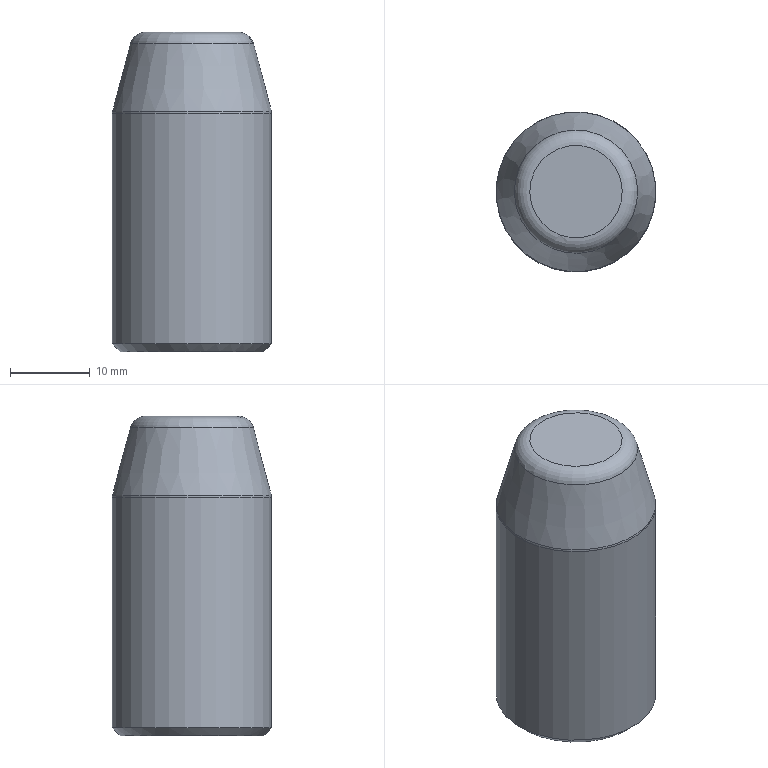Part | STEP file | SN10_014_001_PINO | 1 solid | 9 faces | box 20 x 20 x 40 mm | volume 11102 mm3 | cone 3 | plane 2 | torus 2 | cylinder 2 | commonest cylinder face diameters 6.647 x1 20 x1
STEP:
#1=CARTESIAN_POINT('',(0.,0.,0.));
#2=DIRECTION('',(0.,0.,1.));
#3=DIRECTION('',(1.,0.,0.));
#4=AXIS2_PLACEMENT_3D('',#1,#2,#3);
#5=CARTESIAN_POINT('',(2.917,1.593,47.));
#6=VERTEX_POINT('',#5);
#7=CARTESIAN_POINT('',(0.,0.,47.));
#8=DIRECTION('',(0.,0.,-1.));
#9=DIRECTION('',(1.,0.,0.));
#10=AXIS2_PLACEMENT_3D('',#7,#8,#9);
#11=CIRCLE('',#10,3.324);
#12=CARTESIAN_POINT('',(0.,0.,48.341));
#13=DIRECTION('',(0.,0.,-1.));
#14=DIRECTION('',(0.8776,0.4794,0.));
#15=AXIS2_PLACEMENT_3D('',#12,#13,#14);
#16=CONICAL_SURFACE('',#15,1.,1.047);
#17=CARTESIAN_POINT('',(-5.783,1.341));
#18=DIRECTION('',(1.,0.));
#19=VECTOR('',#18,1.);
#20=LINE('',#17,#19);
#21=(GEOMETRIC_REPRESENTATION_CONTEXT(2)PARAMETRIC_REPRESENTATION_CONTEXT()REPRESENTATION_CONTEXT('',''));
#22=DEFINITIONAL_REPRESENTATION('',(#20),#21);
#23=PCURVE('',#16,#22);
#24=CARTESIAN_POINT('',(0.,0.,29.1));
#25=DIRECTION('',(0.,0.,1.));
#26=DIRECTION('',(0.8776,0.4794,0.));
#27=AXIS2_PLACEMENT_3D('',#24,#25,#26);
#28=CYLINDRICAL_SURFACE('',#27,3.324);
#29=CARTESIAN_POINT('',(12.066,17.9));
#30=DIRECTION('',(-1.,0.));
#31=VECTOR('',#30,1.);
#32=LINE('',#29,#31);
#33=(GEOMETRIC_REPRESENTATION_CONTEXT(2)PARAMETRIC_REPRESENTATION_CONTEXT()REPRESENTATION_CONTEXT('',''));
#34=DEFINITIONAL_REPRESENTATION('',(#32),#33);
#35=PCURVE('',#28,#34);
#36=SURFACE_CURVE('',#11,(#23,#35),.PCURVE_S1.);
#37=EDGE_CURVE('',#6,#6,#36,.T.);
#38=ORIENTED_EDGE('',*,*,#37,.F.);
#39=CARTESIAN_POINT('',(0.,0.,48.919));
#40=VERTEX_POINT('',#39);
#41=CARTESIAN_POINT('',(0.,0.,48.919));
#42=CARTESIAN_POINT('',(2.917,1.593,47.));
#43=B_SPLINE_CURVE_WITH_KNOTS('',1,(#41,#42),.UNSPECIFIED.,.F.,.F.,(2,2),(-1.155,2.683),.PIECEWISE_BEZIER_KNOTS.);
#44=CARTESIAN_POINT('',(0.,0.));
#45=DIRECTION('',(0.,1.));
#46=VECTOR('',#45,1.);
#47=LINE('',#44,#46);
#48=(GEOMETRIC_REPRESENTATION_CONTEXT(2)PARAMETRIC_REPRESENTATION_CONTEXT()REPRESENTATION_CONTEXT('',''));
#49=DEFINITIONAL_REPRESENTATION('',(#47),#48);
#50=PCURVE('',#16,#49);
#51=CARTESIAN_POINT('',(6.283,0.));
#52=DIRECTION('',(0.,1.));
#53=VECTOR('',#52,1.);
#54=LINE('',#51,#53);
#55=(GEOMETRIC_REPRESENTATION_CONTEXT(2)PARAMETRIC_REPRESENTATION_CONTEXT()REPRESENTATION_CONTEXT('',''));
#56=DEFINITIONAL_REPRESENTATION('',(#54),#55);
#57=PCURVE('',#16,#56);
#58=SEAM_CURVE('',#43,(#50,#57),.PCURVE_S1.);
#59=EDGE_CURVE('',#40,#6,#58,.T.);
#60=ORIENTED_EDGE('',*,*,#59,.F.);
#61=ORIENTED_EDGE('',*,*,#59,.T.);
#62=EDGE_LOOP('',(#38,#60,#61));
#63=FACE_BOUND('',#62,.F.);
#64=ADVANCED_FACE('',(#63),#16,.F.);
#65=CARTESIAN_POINT('',(5.078,2.774,69.));
#66=VERTEX_POINT('',#65);
#67=CARTESIAN_POINT('',(0.,0.,69.));
#68=DIRECTION('',(0.,0.,1.));
#69=DIRECTION('',(1.,0.,0.));
#70=AXIS2_PLACEMENT_3D('',#67,#68,#69);
#71=CIRCLE('',#70,5.786);
#72=CARTESIAN_POINT('',(7.321,0.,69.));
#73=DIRECTION('',(0.,0.,1.));
#74=DIRECTION('',(1.,0.,0.));
#75=AXIS2_PLACEMENT_3D('',#72,#73,#74);
#76=PLANE('',#75);
#77=CARTESIAN_POINT('',(-7.321,0.));
#78=DIRECTION('',(1.,0.));
#79=AXIS2_PLACEMENT_2D('',#77,#78);
#80=CIRCLE('',#79,5.786);
#81=(GEOMETRIC_REPRESENTATION_CONTEXT(2)PARAMETRIC_REPRESENTATION_CONTEXT()REPRESENTATION_CONTEXT('',''));
#82=DEFINITIONAL_REPRESENTATION('',(#80),#81);
#83=PCURVE('',#76,#82);
#84=CARTESIAN_POINT('',(0.,0.,67.));
#85=DIRECTION('',(0.,0.,1.));
#86=DIRECTION('',(1.,0.,0.));
#87=AXIS2_PLACEMENT_3D('',#84,#85,#86);
#88=TOROIDAL_SURFACE('',#87,5.786,2.);
#89=CARTESIAN_POINT('',(0.,7.854));
#90=DIRECTION('',(1.,0.));
#91=VECTOR('',#90,1.);
#92=LINE('',#89,#91);
#93=(GEOMETRIC_REPRESENTATION_CONTEXT(2)PARAMETRIC_REPRESENTATION_CONTEXT()REPRESENTATION_CONTEXT('',''));
#94=DEFINITIONAL_REPRESENTATION('',(#92),#93);
#95=PCURVE('',#88,#94);
#96=SURFACE_CURVE('',#71,(#83,#95),.PCURVE_S1.);
#97=EDGE_CURVE('',#66,#66,#96,.T.);
#98=ORIENTED_EDGE('',*,*,#97,.T.);
#99=EDGE_LOOP('',(#98));
#100=FACE_BOUND('',#99,.T.);
#101=ADVANCED_FACE('',(#100),#76,.T.);
#102=ORIENTED_EDGE('',*,*,#97,.F.);
#103=CARTESIAN_POINT('',(6.773,3.7,67.518));
#104=VERTEX_POINT('',#103);
#105=CARTESIAN_POINT('',(6.773,3.7,67.518));
#106=CARTESIAN_POINT('',(6.672,3.645,67.945));
#107=CARTESIAN_POINT('',(6.475,3.537,68.335));
#108=CARTESIAN_POINT('',(6.193,3.383,68.656));
#109=CARTESIAN_POINT('',(5.848,3.195,68.883));
#110=CARTESIAN_POINT('',(5.466,2.986,69.));
#111=CARTESIAN_POINT('',(5.078,2.774,69.));
#112=(BOUNDED_CURVE()B_SPLINE_CURVE(6,(#105,#106,#107,#108,#109,#110,#111),.UNSPECIFIED.,.F.,.F.)B_SPLINE_CURVE_WITH_KNOTS((7,7),(0.2618,1.571),.PIECEWISE_BEZIER_KNOTS.)CURVE()GEOMETRIC_REPRESENTATION_ITEM()RATIONAL_B_SPLINE_CURVE((1.022,1.007,0.9986,0.9958,0.9986,1.007,1.022))REPRESENTATION_ITEM(''));
#113=CARTESIAN_POINT('',(0.5,6.283));
#114=DIRECTION('',(0.,1.));
#115=VECTOR('',#114,1.);
#116=LINE('',#113,#115);
#117=(GEOMETRIC_REPRESENTATION_CONTEXT(2)PARAMETRIC_REPRESENTATION_CONTEXT()REPRESENTATION_CONTEXT('',''));
#118=DEFINITIONAL_REPRESENTATION('',(#116),#117);
#119=PCURVE('',#88,#118);
#120=CARTESIAN_POINT('',(6.783,6.283));
#121=DIRECTION('',(0.,1.));
#122=VECTOR('',#121,1.);
#123=LINE('',#120,#122);
#124=(GEOMETRIC_REPRESENTATION_CONTEXT(2)PARAMETRIC_REPRESENTATION_CONTEXT()REPRESENTATION_CONTEXT('',''));
#125=DEFINITIONAL_REPRESENTATION('',(#123),#124);
#126=PCURVE('',#88,#125);
#127=SEAM_CURVE('',#112,(#119,#126),.PCURVE_S1.);
#128=EDGE_CURVE('',#104,#66,#127,.T.);
#129=ORIENTED_EDGE('',*,*,#128,.F.);
#130=CARTESIAN_POINT('',(0.,0.,67.518));
#131=DIRECTION('',(0.,0.,1.));
#132=DIRECTION('',(1.,0.,0.));
#133=AXIS2_PLACEMENT_3D('',#130,#131,#132);
#134=CIRCLE('',#133,7.718);
#135=CARTESIAN_POINT('',(0.,6.545));
#136=DIRECTION('',(1.,0.));
#137=VECTOR('',#136,1.);
#138=LINE('',#135,#137);
#139=(GEOMETRIC_REPRESENTATION_CONTEXT(2)PARAMETRIC_REPRESENTATION_CONTEXT()REPRESENTATION_CONTEXT('',''));
#140=DEFINITIONAL_REPRESENTATION('',(#138),#139);
#141=PCURVE('',#88,#140);
#142=CARTESIAN_POINT('',(0.,0.,69.));
#143=DIRECTION('',(0.,0.,-1.));
#144=DIRECTION('',(0.8776,0.4794,0.));
#145=AXIS2_PLACEMENT_3D('',#142,#143,#144);
#146=CONICAL_SURFACE('',#145,7.321,0.2618);
#147=CARTESIAN_POINT('',(6.783,1.482));
#148=DIRECTION('',(-1.,0.));
#149=VECTOR('',#148,1.);
#150=LINE('',#147,#149);
#151=(GEOMETRIC_REPRESENTATION_CONTEXT(2)PARAMETRIC_REPRESENTATION_CONTEXT()REPRESENTATION_CONTEXT('',''));
#152=DEFINITIONAL_REPRESENTATION('',(#150),#151);
#153=PCURVE('',#146,#152);
#154=SURFACE_CURVE('',#134,(#141,#153),.PCURVE_S1.);
#155=EDGE_CURVE('',#104,#104,#154,.T.);
#156=ORIENTED_EDGE('',*,*,#155,.T.);
#157=ORIENTED_EDGE('',*,*,#128,.T.);
#158=EDGE_LOOP('',(#102,#129,#156,#157));
#159=FACE_BOUND('',#158,.T.);
#160=ADVANCED_FACE('',(#159),#88,.T.);
#161=CARTESIAN_POINT('',(8.746,4.778,59.127));
#162=VERTEX_POINT('',#161);
#163=CARTESIAN_POINT('',(-8.746,-4.778,59.127));
#164=VERTEX_POINT('',#163);
#165=CARTESIAN_POINT('',(0.,0.,59.127));
#166=DIRECTION('',(0.,0.,-1.));
#167=DIRECTION('',(1.,0.,0.));
#168=AXIS2_PLACEMENT_3D('',#165,#166,#167);
#169=CIRCLE('',#168,9.966);
#170=CARTESIAN_POINT('',(-5.783,9.873));
#171=DIRECTION('',(1.,0.));
#172=VECTOR('',#171,1.);
#173=LINE('',#170,#172);
#174=(GEOMETRIC_REPRESENTATION_CONTEXT(2)PARAMETRIC_REPRESENTATION_CONTEXT()REPRESENTATION_CONTEXT('',''));
#175=DEFINITIONAL_REPRESENTATION('',(#173),#174);
#176=PCURVE('',#146,#175);
#177=CARTESIAN_POINT('',(0.,0.,58.868));
#178=DIRECTION('',(0.,0.,-1.));
#179=DIRECTION('',(-1.,0.,0.));
#180=AXIS2_PLACEMENT_3D('',#177,#178,#179);
#181=TOROIDAL_SURFACE('',#180,9.,1.);
#182=CARTESIAN_POINT('',(-3.142,6.021));
#183=DIRECTION('',(1.,0.));
#184=VECTOR('',#183,1.);
#185=LINE('',#182,#184);
#186=(GEOMETRIC_REPRESENTATION_CONTEXT(2)PARAMETRIC_REPRESENTATION_CONTEXT()REPRESENTATION_CONTEXT('',''));
#187=DEFINITIONAL_REPRESENTATION('',(#185),#186);
#188=PCURVE('',#181,#187);
#189=SURFACE_CURVE('',#169,(#176,#188),.PCURVE_S1.);
#190=EDGE_CURVE('',#162,#164,#189,.T.);
#191=ORIENTED_EDGE('',*,*,#190,.F.);
#192=CARTESIAN_POINT('',(6.773,3.7,67.518));
#193=CARTESIAN_POINT('',(8.746,4.778,59.127));
#194=B_SPLINE_CURVE_WITH_KNOTS('',1,(#192,#193),.UNSPECIFIED.,.F.,.F.,(2,2),(1.535,10.221),.PIECEWISE_BEZIER_KNOTS.);
#195=CARTESIAN_POINT('',(0.,0.));
#196=DIRECTION('',(0.,1.));
#197=VECTOR('',#196,1.);
#198=LINE('',#195,#197);
#199=(GEOMETRIC_REPRESENTATION_CONTEXT(2)PARAMETRIC_REPRESENTATION_CONTEXT()REPRESENTATION_CONTEXT('',''));
#200=DEFINITIONAL_REPRESENTATION('',(#198),#199);
#201=PCURVE('',#146,#200);
#202=CARTESIAN_POINT('',(6.283,0.));
#203=DIRECTION('',(0.,1.));
#204=VECTOR('',#203,1.);
#205=LINE('',#202,#204);
#206=(GEOMETRIC_REPRESENTATION_CONTEXT(2)PARAMETRIC_REPRESENTATION_CONTEXT()REPRESENTATION_CONTEXT('',''));
#207=DEFINITIONAL_REPRESENTATION('',(#205),#206);
#208=PCURVE('',#146,#207);
#209=SEAM_CURVE('',#194,(#201,#208),.PCURVE_S1.);
#210=EDGE_CURVE('',#104,#162,#209,.T.);
#211=ORIENTED_EDGE('',*,*,#210,.F.);
#212=ORIENTED_EDGE('',*,*,#155,.F.);
#213=ORIENTED_EDGE('',*,*,#210,.T.);
#214=CARTESIAN_POINT('',(0.,0.,59.127));
#215=DIRECTION('',(0.,0.,-1.));
#216=DIRECTION('',(1.,0.,0.));
#217=AXIS2_PLACEMENT_3D('',#214,#215,#216);
#218=CIRCLE('',#217,9.966);
#219=CARTESIAN_POINT('',(0.5,9.873));
#220=DIRECTION('',(1.,0.));
#221=VECTOR('',#220,1.);
#222=LINE('',#219,#221);
#223=(GEOMETRIC_REPRESENTATION_CONTEXT(2)PARAMETRIC_REPRESENTATION_CONTEXT()REPRESENTATION_CONTEXT('',''));
#224=DEFINITIONAL_REPRESENTATION('',(#222),#223);
#225=PCURVE('',#146,#224);
#226=CARTESIAN_POINT('',(3.142,6.021));
#227=DIRECTION('',(1.,0.));
#228=VECTOR('',#227,1.);
#229=LINE('',#226,#228);
#230=(GEOMETRIC_REPRESENTATION_CONTEXT(2)PARAMETRIC_REPRESENTATION_CONTEXT()REPRESENTATION_CONTEXT('',''));
#231=DEFINITIONAL_REPRESENTATION('',(#229),#230);
#232=PCURVE('',#181,#231);
#233=SURFACE_CURVE('',#218,(#225,#232),.PCURVE_S1.);
#234=EDGE_CURVE('',#164,#162,#233,.T.);
#235=ORIENTED_EDGE('',*,*,#234,.F.);
#236=EDGE_LOOP('',(#191,#211,#212,#213,#235));
#237=FACE_BOUND('',#236,.T.);
#238=ADVANCED_FACE('',(#237),#146,.T.);
#239=ORIENTED_EDGE('',*,*,#234,.T.);
#240=CARTESIAN_POINT('',(8.776,4.794,58.868));
#241=VERTEX_POINT('',#240);
#242=CARTESIAN_POINT('',(8.746,4.778,59.127));
#243=CARTESIAN_POINT('',(8.756,4.783,59.085));
#244=CARTESIAN_POINT('',(8.764,4.788,59.042));
#245=CARTESIAN_POINT('',(8.77,4.791,58.999));
#246=CARTESIAN_POINT('',(8.774,4.793,58.956));
#247=CARTESIAN_POINT('',(8.776,4.794,58.912));
#248=CARTESIAN_POINT('',(8.776,4.794,58.868));
#249=(BOUNDED_CURVE()B_SPLINE_CURVE(6,(#242,#243,#244,#245,#246,#247,#248),.UNSPECIFIED.,.F.,.F.)B_SPLINE_CURVE_WITH_KNOTS((7,7),(6.021,6.283),.PIECEWISE_BEZIER_KNOTS.)CURVE()GEOMETRIC_REPRESENTATION_ITEM()RATIONAL_B_SPLINE_CURVE((1.001,1.,0.9999,0.9998,0.9999,1.,1.001))REPRESENTATION_ITEM(''));
#250=CARTESIAN_POINT('',(8.925,0.));
#251=DIRECTION('',(0.,1.));
#252=VECTOR('',#251,1.);
#253=LINE('',#250,#252);
#254=(GEOMETRIC_REPRESENTATION_CONTEXT(2)PARAMETRIC_REPRESENTATION_CONTEXT()REPRESENTATION_CONTEXT('',''));
#255=DEFINITIONAL_REPRESENTATION('',(#253),#254);
#256=PCURVE('',#181,#255);
#257=CARTESIAN_POINT('',(2.642,0.));
#258=DIRECTION('',(0.,1.));
#259=VECTOR('',#258,1.);
#260=LINE('',#257,#259);
#261=(GEOMETRIC_REPRESENTATION_CONTEXT(2)PARAMETRIC_REPRESENTATION_CONTEXT()REPRESENTATION_CONTEXT('',''));
#262=DEFINITIONAL_REPRESENTATION('',(#260),#261);
#263=PCURVE('',#181,#262);
#264=SEAM_CURVE('',#249,(#256,#263),.PCURVE_S1.);
#265=EDGE_CURVE('',#162,#241,#264,.T.);
#266=ORIENTED_EDGE('',*,*,#265,.T.);
#267=CARTESIAN_POINT('',(0.,0.,58.868));
#268=DIRECTION('',(0.,0.,-1.));
#269=DIRECTION('',(1.,0.,0.));
#270=AXIS2_PLACEMENT_3D('',#267,#268,#269);
#271=CIRCLE('',#270,10.);
#272=CARTESIAN_POINT('',(-3.142,6.283));
#273=DIRECTION('',(1.,0.));
#274=VECTOR('',#273,1.);
#275=LINE('',#272,#274);
#276=(GEOMETRIC_REPRESENTATION_CONTEXT(2)PARAMETRIC_REPRESENTATION_CONTEXT()REPRESENTATION_CONTEXT('',''));
#277=DEFINITIONAL_REPRESENTATION('',(#275),#276);
#278=PCURVE('',#181,#277);
#279=CARTESIAN_POINT('',(0.,0.,49.));
#280=DIRECTION('',(0.,0.,1.));
#281=DIRECTION('',(0.8776,0.4794,0.));
#282=AXIS2_PLACEMENT_3D('',#279,#280,#281);
#283=CYLINDRICAL_SURFACE('',#282,10.);
#284=CARTESIAN_POINT('',(12.066,9.868));
#285=DIRECTION('',(-1.,0.));
#286=VECTOR('',#285,1.);
#287=LINE('',#284,#286);
#288=(GEOMETRIC_REPRESENTATION_CONTEXT(2)PARAMETRIC_REPRESENTATION_CONTEXT()REPRESENTATION_CONTEXT('',''));
#289=DEFINITIONAL_REPRESENTATION('',(#287),#288);
#290=PCURVE('',#283,#289);
#291=SURFACE_CURVE('',#271,(#278,#290),.PCURVE_S1.);
#292=EDGE_CURVE('',#241,#241,#291,.T.);
#293=ORIENTED_EDGE('',*,*,#292,.F.);
#294=ORIENTED_EDGE('',*,*,#265,.F.);
#295=ORIENTED_EDGE('',*,*,#190,.T.);
#296=EDGE_LOOP('',(#239,#266,#293,#294,#295));
#297=FACE_BOUND('',#296,.T.);
#298=ADVANCED_FACE('',(#297),#181,.T.);
#299=CARTESIAN_POINT('',(-8.776,-4.794,30.));
#300=VERTEX_POINT('',#299);
#301=CARTESIAN_POINT('',(8.776,4.794,30.));
#302=VERTEX_POINT('',#301);
#303=CARTESIAN_POINT('',(0.,0.,30.));
#304=DIRECTION('',(0.,0.,1.));
#305=DIRECTION('',(1.,0.,0.));
#306=AXIS2_PLACEMENT_3D('',#303,#304,#305);
#307=CIRCLE('',#306,10.);
#308=CARTESIAN_POINT('',(-0.5,-19.));
#309=DIRECTION('',(1.,0.));
#310=VECTOR('',#309,1.);
#311=LINE('',#308,#310);
#312=(GEOMETRIC_REPRESENTATION_CONTEXT(2)PARAMETRIC_REPRESENTATION_CONTEXT()REPRESENTATION_CONTEXT('',''));
#313=DEFINITIONAL_REPRESENTATION('',(#311),#312);
#314=PCURVE('',#283,#313);
#315=CARTESIAN_POINT('',(0.,0.,21.));
#316=DIRECTION('',(0.,0.,1.));
#317=DIRECTION('',(-0.9409,-0.3387,0.));
#318=AXIS2_PLACEMENT_3D('',#315,#316,#317);
#319=CONICAL_SURFACE('',#318,1.,0.7854);
#320=CARTESIAN_POINT('',(2.796,9.));
#321=DIRECTION('',(1.,0.));
#322=VECTOR('',#321,1.);
#323=LINE('',#320,#322);
#324=(GEOMETRIC_REPRESENTATION_CONTEXT(2)PARAMETRIC_REPRESENTATION_CONTEXT()REPRESENTATION_CONTEXT('',''));
#325=DEFINITIONAL_REPRESENTATION('',(#323),#324);
#326=PCURVE('',#319,#325);
#327=SURFACE_CURVE('',#307,(#314,#326),.PCURVE_S1.);
#328=EDGE_CURVE('',#300,#302,#327,.T.);
#329=ORIENTED_EDGE('',*,*,#328,.T.);
#330=CARTESIAN_POINT('',(8.776,4.794,30.));
#331=CARTESIAN_POINT('',(8.776,4.794,58.868));
#332=B_SPLINE_CURVE_WITH_KNOTS('',1,(#330,#331),.UNSPECIFIED.,.F.,.F.,(2,2),(-19.,9.868),.PIECEWISE_BEZIER_KNOTS.);
#333=CARTESIAN_POINT('',(6.283,0.));
#334=DIRECTION('',(0.,1.));
#335=VECTOR('',#334,1.);
#336=LINE('',#333,#335);
#337=(GEOMETRIC_REPRESENTATION_CONTEXT(2)PARAMETRIC_REPRESENTATION_CONTEXT()REPRESENTATION_CONTEXT('',''));
#338=DEFINITIONAL_REPRESENTATION('',(#336),#337);
#339=PCURVE('',#283,#338);
#340=CARTESIAN_POINT('',(0.,0.));
#341=DIRECTION('',(0.,1.));
#342=VECTOR('',#341,1.);
#343=LINE('',#340,#342);
#344=(GEOMETRIC_REPRESENTATION_CONTEXT(2)PARAMETRIC_REPRESENTATION_CONTEXT()REPRESENTATION_CONTEXT('',''));
#345=DEFINITIONAL_REPRESENTATION('',(#343),#344);
#346=PCURVE('',#283,#345);
#347=SEAM_CURVE('',#332,(#339,#346),.PCURVE_S1.);
#348=EDGE_CURVE('',#302,#241,#347,.T.);
#349=ORIENTED_EDGE('',*,*,#348,.T.);
#350=ORIENTED_EDGE('',*,*,#292,.T.);
#351=ORIENTED_EDGE('',*,*,#348,.F.);
#352=CARTESIAN_POINT('',(0.,0.,30.));
#353=DIRECTION('',(0.,0.,1.));
#354=DIRECTION('',(1.,0.,0.));
#355=AXIS2_PLACEMENT_3D('',#352,#353,#354);
#356=CIRCLE('',#355,10.);
#357=CARTESIAN_POINT('',(-0.5,-19.));
#358=DIRECTION('',(1.,0.));
#359=VECTOR('',#358,1.);
#360=LINE('',#357,#359);
#361=(GEOMETRIC_REPRESENTATION_CONTEXT(2)PARAMETRIC_REPRESENTATION_CONTEXT()REPRESENTATION_CONTEXT('',''));
#362=DEFINITIONAL_REPRESENTATION('',(#360),#361);
#363=PCURVE('',#283,#362);
#364=CARTESIAN_POINT('',(2.796,9.));
#365=DIRECTION('',(1.,0.));
#366=VECTOR('',#365,1.);
#367=LINE('',#364,#366);
#368=(GEOMETRIC_REPRESENTATION_CONTEXT(2)PARAMETRIC_REPRESENTATION_CONTEXT()REPRESENTATION_CONTEXT('',''));
#369=DEFINITIONAL_REPRESENTATION('',(#367),#368);
#370=PCURVE('',#319,#369);
#371=SURFACE_CURVE('',#356,(#363,#370),.PCURVE_S1.);
#372=EDGE_CURVE('',#302,#300,#371,.T.);
#373=ORIENTED_EDGE('',*,*,#372,.T.);
#374=EDGE_LOOP('',(#329,#349,#350,#351,#373));
#375=FACE_BOUND('',#374,.T.);
#376=ADVANCED_FACE('',(#375),#283,.T.);
#377=ORIENTED_EDGE('',*,*,#328,.F.);
#378=ORIENTED_EDGE('',*,*,#372,.F.);
#379=CARTESIAN_POINT('',(7.898,4.315,29.));
#380=VERTEX_POINT('',#379);
#381=CARTESIAN_POINT('',(7.898,4.315,29.));
#382=CARTESIAN_POINT('',(8.776,4.794,30.));
#383=B_SPLINE_CURVE_WITH_KNOTS('',1,(#381,#382),.UNSPECIFIED.,.F.,.F.,(2,2),(11.314,12.728),.PIECEWISE_BEZIER_KNOTS.);
#384=CARTESIAN_POINT('',(3.296,0.));
#385=DIRECTION('',(0.,1.));
#386=VECTOR('',#385,1.);
#387=LINE('',#384,#386);
#388=(GEOMETRIC_REPRESENTATION_CONTEXT(2)PARAMETRIC_REPRESENTATION_CONTEXT()REPRESENTATION_CONTEXT('',''));
#389=DEFINITIONAL_REPRESENTATION('',(#387),#388);
#390=PCURVE('',#319,#389);
#391=CARTESIAN_POINT('',(9.579,0.));
#392=DIRECTION('',(0.,1.));
#393=VECTOR('',#392,1.);
#394=LINE('',#391,#393);
#395=(GEOMETRIC_REPRESENTATION_CONTEXT(2)PARAMETRIC_REPRESENTATION_CONTEXT()REPRESENTATION_CONTEXT('',''));
#396=DEFINITIONAL_REPRESENTATION('',(#394),#395);
#397=PCURVE('',#319,#396);
#398=SEAM_CURVE('',#383,(#390,#397),.PCURVE_S1.);
#399=EDGE_CURVE('',#380,#302,#398,.T.);
#400=ORIENTED_EDGE('',*,*,#399,.F.);
#401=CARTESIAN_POINT('',(0.,0.,29.));
#402=DIRECTION('',(0.,0.,1.));
#403=DIRECTION('',(1.,0.,0.));
#404=AXIS2_PLACEMENT_3D('',#401,#402,#403);
#405=CIRCLE('',#404,9.);
#406=CARTESIAN_POINT('',(2.796,8.));
#407=DIRECTION('',(1.,0.));
#408=VECTOR('',#407,1.);
#409=LINE('',#406,#408);
#410=(GEOMETRIC_REPRESENTATION_CONTEXT(2)PARAMETRIC_REPRESENTATION_CONTEXT()REPRESENTATION_CONTEXT('',''));
#411=DEFINITIONAL_REPRESENTATION('',(#409),#410);
#412=PCURVE('',#319,#411);
#413=CARTESIAN_POINT('',(0.,0.,29.));
#414=DIRECTION('',(0.,0.,1.));
#415=DIRECTION('',(1.,0.,0.));
#416=AXIS2_PLACEMENT_3D('',#413,#414,#415);
#417=PLANE('',#416);
#418=CARTESIAN_POINT('',(0.,0.));
#419=DIRECTION('',(1.,0.));
#420=AXIS2_PLACEMENT_2D('',#418,#419);
#421=CIRCLE('',#420,9.);
#422=(GEOMETRIC_REPRESENTATION_CONTEXT(2)PARAMETRIC_REPRESENTATION_CONTEXT()REPRESENTATION_CONTEXT('',''));
#423=DEFINITIONAL_REPRESENTATION('',(#421),#422);
#424=PCURVE('',#417,#423);
#425=SURFACE_CURVE('',#405,(#412,#424),.PCURVE_S1.);
#426=EDGE_CURVE('',#380,#380,#425,.T.);
#427=ORIENTED_EDGE('',*,*,#426,.T.);
#428=ORIENTED_EDGE('',*,*,#399,.T.);
#429=EDGE_LOOP('',(#377,#378,#400,#427,#428));
#430=FACE_BOUND('',#429,.T.);
#431=ADVANCED_FACE('',(#430),#319,.T.);
#432=ORIENTED_EDGE('',*,*,#426,.F.);
#433=EDGE_LOOP('',(#432));
#434=FACE_BOUND('',#433,.T.);
#435=CARTESIAN_POINT('',(2.917,1.593,29.));
#436=VERTEX_POINT('',#435);
#437=CARTESIAN_POINT('',(0.,0.,29.));
#438=DIRECTION('',(0.,0.,1.));
#439=DIRECTION('',(1.,0.,0.));
#440=AXIS2_PLACEMENT_3D('',#437,#438,#439);
#441=CIRCLE('',#440,3.324);
#442=CARTESIAN_POINT('',(0.,0.));
#443=DIRECTION('',(1.,0.));
#444=AXIS2_PLACEMENT_2D('',#442,#443);
#445=CIRCLE('',#444,3.324);
#446=(GEOMETRIC_REPRESENTATION_CONTEXT(2)PARAMETRIC_REPRESENTATION_CONTEXT()REPRESENTATION_CONTEXT('',''));
#447=DEFINITIONAL_REPRESENTATION('',(#445),#446);
#448=PCURVE('',#417,#447);
#449=CARTESIAN_POINT('',(-0.5,-0.1));
#450=DIRECTION('',(1.,0.));
#451=VECTOR('',#450,1.);
#452=LINE('',#449,#451);
#453=(GEOMETRIC_REPRESENTATION_CONTEXT(2)PARAMETRIC_REPRESENTATION_CONTEXT()REPRESENTATION_CONTEXT('',''));
#454=DEFINITIONAL_REPRESENTATION('',(#452),#453);
#455=PCURVE('',#28,#454);
#456=SURFACE_CURVE('',#441,(#448,#455),.PCURVE_S1.);
#457=EDGE_CURVE('',#436,#436,#456,.T.);
#458=ORIENTED_EDGE('',*,*,#457,.T.);
#459=EDGE_LOOP('',(#458));
#460=FACE_BOUND('',#459,.T.);
#461=ADVANCED_FACE('',(#434,#460),#417,.F.);
#462=ORIENTED_EDGE('',*,*,#457,.T.);
#463=CARTESIAN_POINT('',(2.917,1.593,29.));
#464=CARTESIAN_POINT('',(2.917,1.593,47.));
#465=B_SPLINE_CURVE_WITH_KNOTS('',1,(#463,#464),.UNSPECIFIED.,.F.,.F.,(2,2),(-0.1,17.9),.PIECEWISE_BEZIER_KNOTS.);
#466=CARTESIAN_POINT('',(6.283,0.));
#467=DIRECTION('',(0.,1.));
#468=VECTOR('',#467,1.);
#469=LINE('',#466,#468);
#470=(GEOMETRIC_REPRESENTATION_CONTEXT(2)PARAMETRIC_REPRESENTATION_CONTEXT()REPRESENTATION_CONTEXT('',''));
#471=DEFINITIONAL_REPRESENTATION('',(#469),#470);
#472=PCURVE('',#28,#471);
#473=CARTESIAN_POINT('',(0.,0.));
#474=DIRECTION('',(0.,1.));
#475=VECTOR('',#474,1.);
#476=LINE('',#473,#475);
#477=(GEOMETRIC_REPRESENTATION_CONTEXT(2)PARAMETRIC_REPRESENTATION_CONTEXT()REPRESENTATION_CONTEXT('',''));
#478=DEFINITIONAL_REPRESENTATION('',(#476),#477);
#479=PCURVE('',#28,#478);
#480=SEAM_CURVE('',#465,(#472,#479),.PCURVE_S1.);
#481=EDGE_CURVE('',#436,#6,#480,.T.);
#482=ORIENTED_EDGE('',*,*,#481,.T.);
#483=ORIENTED_EDGE('',*,*,#37,.T.);
#484=ORIENTED_EDGE('',*,*,#481,.F.);
#485=EDGE_LOOP('',(#462,#482,#483,#484));
#486=FACE_BOUND('',#485,.F.);
#487=ADVANCED_FACE('',(#486),#28,.F.);
#488=CLOSED_SHELL('',(#64,#101,#160,#238,#298,#376,#431,#461,#487));
#489=MANIFOLD_SOLID_BREP('',#488);
#490=(LENGTH_UNIT()NAMED_UNIT(*)SI_UNIT(.MILLI.,.METRE.));
#491=UNCERTAINTY_MEASURE_WITH_UNIT(LENGTH_MEASURE(0.00001),#490,'','');
#492=(NAMED_UNIT(*)PLANE_ANGLE_UNIT()SI_UNIT($,.RADIAN.));
#493=(NAMED_UNIT(*)SI_UNIT($,.STERADIAN.)SOLID_ANGLE_UNIT());
#494=(GEOMETRIC_REPRESENTATION_CONTEXT(3)GLOBAL_UNCERTAINTY_ASSIGNED_CONTEXT((#491))GLOBAL_UNIT_ASSIGNED_CONTEXT((#490,#492,#493))REPRESENTATION_CONTEXT('',''));
#495=ADVANCED_BREP_SHAPE_REPRESENTATION('',(#4,#489),#494);